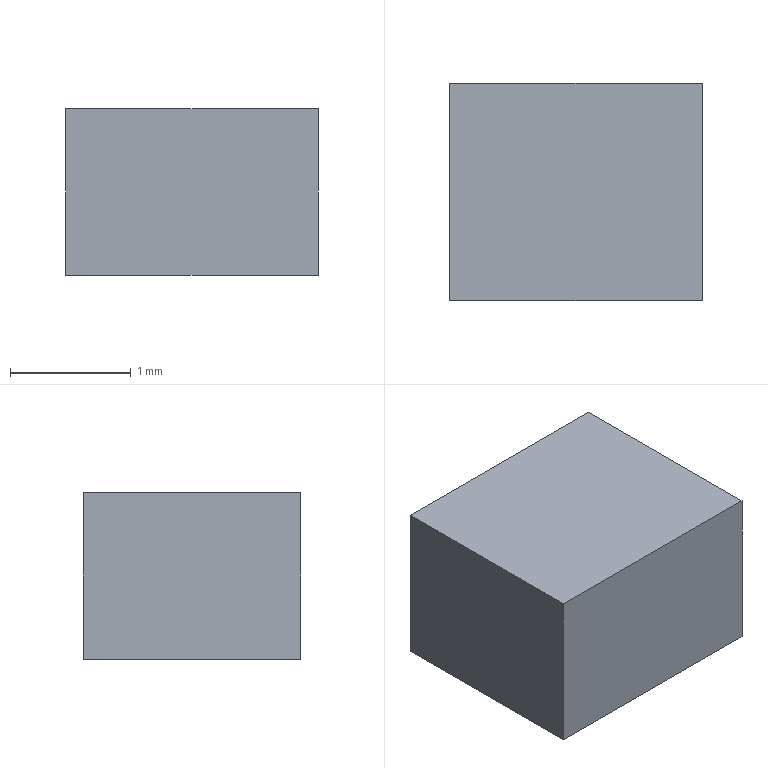Part | Creo | 1 solid | 6 faces | box 2.094 x 1.8 x 1.381 mm | volume 5.204 mm3 | plane 6
STEP:
#1=CARTESIAN_POINT('',(0.,0.,0.));
#2=DIRECTION('',(0.,0.,1.));
#3=DIRECTION('',(1.,0.,0.));
#4=AXIS2_PLACEMENT_3D('',#1,#2,#3);
#5=CARTESIAN_POINT('',(-1.194,-0.9,0.));
#6=VERTEX_POINT('',#5);
#7=CARTESIAN_POINT('',(0.9,-0.9,0.));
#8=VERTEX_POINT('',#7);
#9=CARTESIAN_POINT('',(-1.194,-0.9,0.));
#10=DIRECTION('',(1.,0.,0.));
#11=VECTOR('',#10,2.094);
#12=LINE('',#9,#11);
#13=EDGE_CURVE('',#6,#8,#12,.T.);
#14=ORIENTED_EDGE('',*,*,#13,.T.);
#15=CARTESIAN_POINT('',(0.9,0.9,0.));
#16=VERTEX_POINT('',#15);
#17=CARTESIAN_POINT('',(0.9,-0.9,0.));
#18=DIRECTION('',(0.,1.,0.));
#19=VECTOR('',#18,1.8);
#20=LINE('',#17,#19);
#21=EDGE_CURVE('',#8,#16,#20,.T.);
#22=ORIENTED_EDGE('',*,*,#21,.T.);
#23=CARTESIAN_POINT('',(-1.194,0.9,0.));
#24=VERTEX_POINT('',#23);
#25=CARTESIAN_POINT('',(0.9,0.9,0.));
#26=DIRECTION('',(-1.,0.,0.));
#27=VECTOR('',#26,2.094);
#28=LINE('',#25,#27);
#29=EDGE_CURVE('',#16,#24,#28,.T.);
#30=ORIENTED_EDGE('',*,*,#29,.T.);
#31=CARTESIAN_POINT('',(-1.194,0.9,0.));
#32=DIRECTION('',(0.,-1.,0.));
#33=VECTOR('',#32,1.8);
#34=LINE('',#31,#33);
#35=EDGE_CURVE('',#24,#6,#34,.T.);
#36=ORIENTED_EDGE('',*,*,#35,.T.);
#37=EDGE_LOOP('',(#14,#22,#30,#36));
#38=FACE_OUTER_BOUND('',#37,.F.);
#39=CARTESIAN_POINT('',(0.,0.,0.));
#40=DIRECTION('',(0.,0.,1.));
#41=DIRECTION('',(1.,0.,0.));
#42=AXIS2_PLACEMENT_3D('',#39,#40,#41);
#43=PLANE('',#42);
#44=ADVANCED_FACE('',(#38),#43,.F.);
#45=ORIENTED_EDGE('',*,*,#13,.F.);
#46=CARTESIAN_POINT('',(-1.194,-0.9,1.381));
#47=VERTEX_POINT('',#46);
#48=CARTESIAN_POINT('',(-1.194,-0.9,0.));
#49=DIRECTION('',(0.,0.,1.));
#50=VECTOR('',#49,1.381);
#51=LINE('',#48,#50);
#52=EDGE_CURVE('',#6,#47,#51,.T.);
#53=ORIENTED_EDGE('',*,*,#52,.T.);
#54=CARTESIAN_POINT('',(0.9,-0.9,1.381));
#55=VERTEX_POINT('',#54);
#56=CARTESIAN_POINT('',(-1.194,-0.9,1.381));
#57=DIRECTION('',(1.,0.,0.));
#58=VECTOR('',#57,2.094);
#59=LINE('',#56,#58);
#60=EDGE_CURVE('',#47,#55,#59,.T.);
#61=ORIENTED_EDGE('',*,*,#60,.T.);
#62=CARTESIAN_POINT('',(0.9,-0.9,0.));
#63=DIRECTION('',(0.,0.,1.));
#64=VECTOR('',#63,1.381);
#65=LINE('',#62,#64);
#66=EDGE_CURVE('',#8,#55,#65,.T.);
#67=ORIENTED_EDGE('',*,*,#66,.F.);
#68=EDGE_LOOP('',(#45,#53,#61,#67));
#69=FACE_OUTER_BOUND('',#68,.F.);
#70=CARTESIAN_POINT('',(-1.194,-0.9,0.));
#71=DIRECTION('',(0.,-1.,0.));
#72=DIRECTION('',(1.,0.,0.));
#73=AXIS2_PLACEMENT_3D('',#70,#71,#72);
#74=PLANE('',#73);
#75=ADVANCED_FACE('',(#69),#74,.T.);
#76=ORIENTED_EDGE('',*,*,#35,.F.);
#77=CARTESIAN_POINT('',(-1.194,0.9,1.381));
#78=VERTEX_POINT('',#77);
#79=CARTESIAN_POINT('',(-1.194,0.9,0.));
#80=DIRECTION('',(0.,0.,1.));
#81=VECTOR('',#80,1.381);
#82=LINE('',#79,#81);
#83=EDGE_CURVE('',#24,#78,#82,.T.);
#84=ORIENTED_EDGE('',*,*,#83,.T.);
#85=CARTESIAN_POINT('',(-1.194,0.9,1.381));
#86=DIRECTION('',(0.,-1.,0.));
#87=VECTOR('',#86,1.8);
#88=LINE('',#85,#87);
#89=EDGE_CURVE('',#78,#47,#88,.T.);
#90=ORIENTED_EDGE('',*,*,#89,.T.);
#91=ORIENTED_EDGE('',*,*,#52,.F.);
#92=EDGE_LOOP('',(#76,#84,#90,#91));
#93=FACE_OUTER_BOUND('',#92,.F.);
#94=CARTESIAN_POINT('',(-1.194,0.9,0.));
#95=DIRECTION('',(-1.,0.,0.));
#96=DIRECTION('',(0.,-1.,0.));
#97=AXIS2_PLACEMENT_3D('',#94,#95,#96);
#98=PLANE('',#97);
#99=ADVANCED_FACE('',(#93),#98,.T.);
#100=ORIENTED_EDGE('',*,*,#29,.F.);
#101=CARTESIAN_POINT('',(0.9,0.9,1.381));
#102=VERTEX_POINT('',#101);
#103=CARTESIAN_POINT('',(0.9,0.9,0.));
#104=DIRECTION('',(0.,0.,1.));
#105=VECTOR('',#104,1.381);
#106=LINE('',#103,#105);
#107=EDGE_CURVE('',#16,#102,#106,.T.);
#108=ORIENTED_EDGE('',*,*,#107,.T.);
#109=CARTESIAN_POINT('',(0.9,0.9,1.381));
#110=DIRECTION('',(-1.,0.,0.));
#111=VECTOR('',#110,2.094);
#112=LINE('',#109,#111);
#113=EDGE_CURVE('',#102,#78,#112,.T.);
#114=ORIENTED_EDGE('',*,*,#113,.T.);
#115=ORIENTED_EDGE('',*,*,#83,.F.);
#116=EDGE_LOOP('',(#100,#108,#114,#115));
#117=FACE_OUTER_BOUND('',#116,.F.);
#118=CARTESIAN_POINT('',(0.9,0.9,0.));
#119=DIRECTION('',(0.,1.,0.));
#120=DIRECTION('',(-1.,0.,0.));
#121=AXIS2_PLACEMENT_3D('',#118,#119,#120);
#122=PLANE('',#121);
#123=ADVANCED_FACE('',(#117),#122,.T.);
#124=ORIENTED_EDGE('',*,*,#21,.F.);
#125=ORIENTED_EDGE('',*,*,#66,.T.);
#126=CARTESIAN_POINT('',(0.9,-0.9,1.381));
#127=DIRECTION('',(0.,1.,0.));
#128=VECTOR('',#127,1.8);
#129=LINE('',#126,#128);
#130=EDGE_CURVE('',#55,#102,#129,.T.);
#131=ORIENTED_EDGE('',*,*,#130,.T.);
#132=ORIENTED_EDGE('',*,*,#107,.F.);
#133=EDGE_LOOP('',(#124,#125,#131,#132));
#134=FACE_OUTER_BOUND('',#133,.F.);
#135=CARTESIAN_POINT('',(0.9,-0.9,0.));
#136=DIRECTION('',(1.,0.,0.));
#137=DIRECTION('',(0.,1.,0.));
#138=AXIS2_PLACEMENT_3D('',#135,#136,#137);
#139=PLANE('',#138);
#140=ADVANCED_FACE('',(#134),#139,.T.);
#141=ORIENTED_EDGE('',*,*,#60,.F.);
#142=ORIENTED_EDGE('',*,*,#89,.F.);
#143=ORIENTED_EDGE('',*,*,#113,.F.);
#144=ORIENTED_EDGE('',*,*,#130,.F.);
#145=EDGE_LOOP('',(#141,#142,#143,#144));
#146=FACE_OUTER_BOUND('',#145,.F.);
#147=CARTESIAN_POINT('',(0.,0.,1.381));
#148=DIRECTION('',(0.,0.,1.));
#149=DIRECTION('',(1.,0.,0.));
#150=AXIS2_PLACEMENT_3D('',#147,#148,#149);
#151=PLANE('',#150);
#152=ADVANCED_FACE('',(#146),#151,.T.);
#153=CLOSED_SHELL('',(#44,#75,#99,#123,#140,#152));
#154=MANIFOLD_SOLID_BREP('',#153);
#155=(LENGTH_UNIT()NAMED_UNIT(*)SI_UNIT(.MILLI.,.METRE.));
#156=UNCERTAINTY_MEASURE_WITH_UNIT(LENGTH_MEASURE(0.0003087),#155,'','');
#157=(NAMED_UNIT(*)PLANE_ANGLE_UNIT()SI_UNIT($,.RADIAN.));
#158=PLANE_ANGLE_MEASURE_WITH_UNIT(PLANE_ANGLE_MEASURE(0.01745),#157);
#159=(CONVERSION_BASED_UNIT('DEGREE',#158)NAMED_UNIT(*)PLANE_ANGLE_UNIT());
#160=(NAMED_UNIT(*)SI_UNIT($,.STERADIAN.)SOLID_ANGLE_UNIT());
#161=(GEOMETRIC_REPRESENTATION_CONTEXT(3)GLOBAL_UNCERTAINTY_ASSIGNED_CONTEXT((#156))GLOBAL_UNIT_ASSIGNED_CONTEXT((#155,#159,#160))REPRESENTATION_CONTEXT('',''));
#162=ADVANCED_BREP_SHAPE_REPRESENTATION('',(#4,#154),#161);